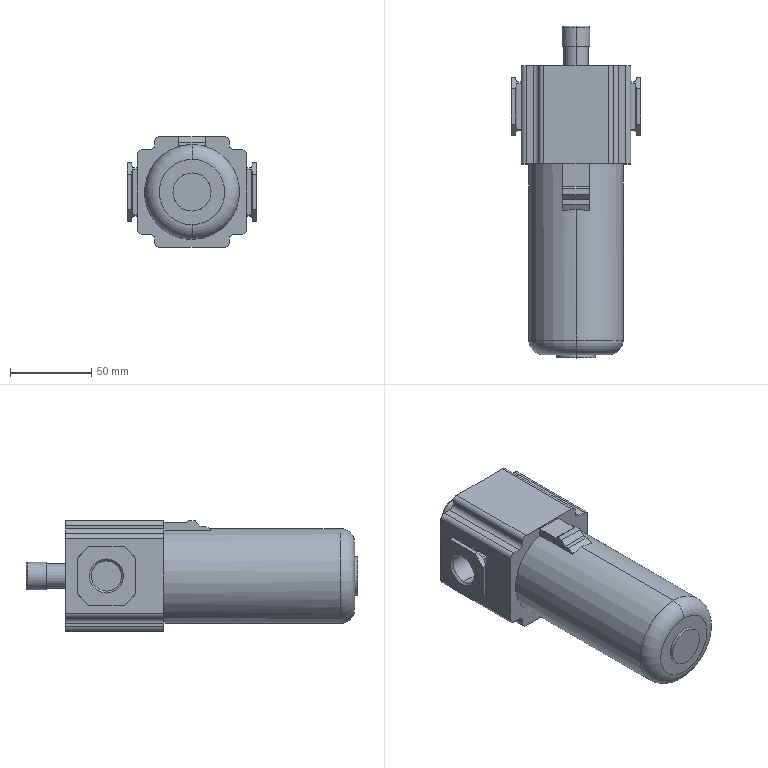Part | SolidWorks | features BaseBody 1 | 1 solid | 106 faces | box 80 x 204.5 x 68 mm | volume 577118 mm3 | plane 72 | cylinder 26 | torus 4 | cone 4 | commonest cylinder face diameters 6 x12 18.631 x4 11.8 x2 15 x2 17 x2 23.5 x2